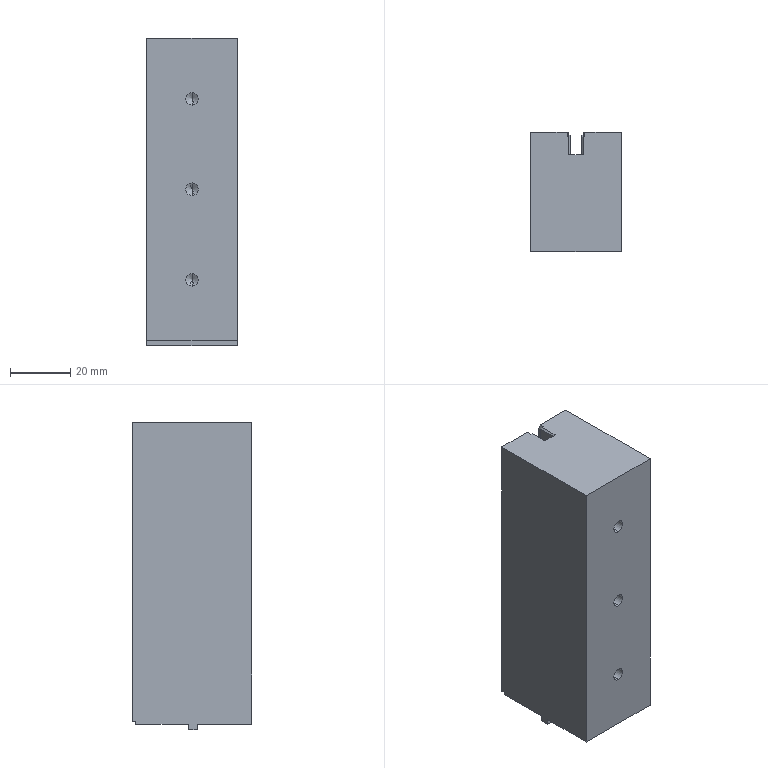Part | STEP file | Rivet feed slide_Default | 1 solid | 70 faces | box 30 x 39.6 x 101.8 mm | volume 114670 mm3 | plane 26 | cylinder 22 | cone 22 | commonest cylinder face diameters 2.5 x12 4.2 x10